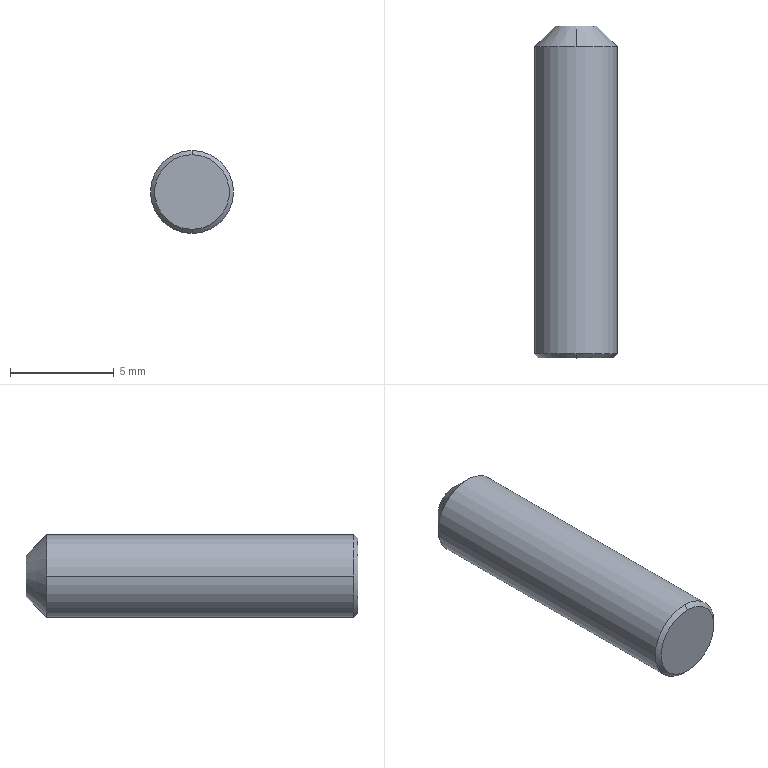Part | STEP file | 1 solid | 8 faces | box 4 x 16 x 4 mm | volume 195.583 mm3 | cone 4 | cylinder 2 | plane 2 | commonest cylinder face diameters 4 x2
STEP:
#1=CARTESIAN_POINT('',(0.,0.,0.));
#2=DIRECTION('',(0.,0.,1.));
#3=DIRECTION('',(1.,0.,0.));
#4=AXIS2_PLACEMENT_3D('',#1,#2,#3);
#5=CARTESIAN_POINT('',(0.,0.,-1.8));
#6=VERTEX_POINT('',#5);
#7=CARTESIAN_POINT('',(0.,0.,1.8));
#8=VERTEX_POINT('',#7);
#9=CARTESIAN_POINT('',(0.,0.,0.));
#10=DIRECTION('',(0.,-1.,0.));
#11=DIRECTION('',(0.,0.,1.));
#12=AXIS2_PLACEMENT_3D('',#9,#10,#11);
#13=CIRCLE('',#12,1.8);
#14=CARTESIAN_POINT('',(0.,0.,0.));
#15=DIRECTION('',(0.,1.,0.));
#16=DIRECTION('',(0.,0.,1.));
#17=AXIS2_PLACEMENT_3D('',#14,#15,#16);
#18=CONICAL_SURFACE('',#17,1.8,0.7854);
#19=CARTESIAN_POINT('',(6.283,0.));
#20=DIRECTION('',(-1.,0.));
#21=VECTOR('',#20,1.);
#22=LINE('',#19,#21);
#23=(GEOMETRIC_REPRESENTATION_CONTEXT(2)PARAMETRIC_REPRESENTATION_CONTEXT()REPRESENTATION_CONTEXT('',''));
#24=DEFINITIONAL_REPRESENTATION('',(#22),#23);
#25=PCURVE('',#18,#24);
#26=CARTESIAN_POINT('',(-1.822,0.,1.822));
#27=DIRECTION('',(0.,-1.,0.));
#28=DIRECTION('',(0.,0.,-1.));
#29=AXIS2_PLACEMENT_3D('',#26,#27,#28);
#30=PLANE('',#29);
#31=CARTESIAN_POINT('',(1.822,1.822));
#32=DIRECTION('',(-1.,0.));
#33=AXIS2_PLACEMENT_2D('',#31,#32);
#34=CIRCLE('',#33,1.8);
#35=(GEOMETRIC_REPRESENTATION_CONTEXT(2)PARAMETRIC_REPRESENTATION_CONTEXT()REPRESENTATION_CONTEXT('',''));
#36=DEFINITIONAL_REPRESENTATION('',(#34),#35);
#37=PCURVE('',#30,#36);
#38=SURFACE_CURVE('',#13,(#25,#37),.PCURVE_S1.);
#39=EDGE_CURVE('',#6,#8,#38,.T.);
#40=ORIENTED_EDGE('',*,*,#39,.F.);
#41=CARTESIAN_POINT('',(0.,0.2,-2.));
#42=VERTEX_POINT('',#41);
#43=CARTESIAN_POINT('',(0.,0.,-1.8));
#44=DIRECTION('',(0.,0.7071,-0.7071));
#45=VECTOR('',#44,1.);
#46=LINE('',#43,#45);
#47=CARTESIAN_POINT('',(3.142,0.));
#48=DIRECTION('',(0.,1.));
#49=VECTOR('',#48,1.);
#50=LINE('',#47,#49);
#51=(GEOMETRIC_REPRESENTATION_CONTEXT(2)PARAMETRIC_REPRESENTATION_CONTEXT()REPRESENTATION_CONTEXT('',''));
#52=DEFINITIONAL_REPRESENTATION('',(#50),#51);
#53=PCURVE('',#18,#52);
#54=CARTESIAN_POINT('',(0.,0.,0.));
#55=DIRECTION('',(0.,1.,0.));
#56=DIRECTION('',(0.,0.,1.));
#57=AXIS2_PLACEMENT_3D('',#54,#55,#56);
#58=CONICAL_SURFACE('',#57,1.8,0.7854);
#59=CARTESIAN_POINT('',(3.142,0.));
#60=DIRECTION('',(0.,1.));
#61=VECTOR('',#60,1.);
#62=LINE('',#59,#61);
#63=(GEOMETRIC_REPRESENTATION_CONTEXT(2)PARAMETRIC_REPRESENTATION_CONTEXT()REPRESENTATION_CONTEXT('',''));
#64=DEFINITIONAL_REPRESENTATION('',(#62),#63);
#65=PCURVE('',#58,#64);
#66=SURFACE_CURVE('',#46,(#53,#65),.PCURVE_S1.);
#67=EDGE_CURVE('',#6,#42,#66,.T.);
#68=ORIENTED_EDGE('',*,*,#67,.T.);
#69=CARTESIAN_POINT('',(2.,0.2,0.));
#70=VERTEX_POINT('',#69);
#71=CARTESIAN_POINT('',(0.,0.2,0.));
#72=DIRECTION('',(0.,1.,0.));
#73=DIRECTION('',(0.,0.,1.));
#74=AXIS2_PLACEMENT_3D('',#71,#72,#73);
#75=CIRCLE('',#74,2.);
#76=CARTESIAN_POINT('',(0.,0.2));
#77=DIRECTION('',(1.,0.));
#78=VECTOR('',#77,1.);
#79=LINE('',#76,#78);
#80=(GEOMETRIC_REPRESENTATION_CONTEXT(2)PARAMETRIC_REPRESENTATION_CONTEXT()REPRESENTATION_CONTEXT('',''));
#81=DEFINITIONAL_REPRESENTATION('',(#79),#80);
#82=PCURVE('',#18,#81);
#83=CARTESIAN_POINT('',(0.,15.,0.));
#84=DIRECTION('',(0.,-1.,0.));
#85=DIRECTION('',(1.,0.,0.));
#86=AXIS2_PLACEMENT_3D('',#83,#84,#85);
#87=CYLINDRICAL_SURFACE('',#86,2.);
#88=CARTESIAN_POINT('',(7.854,14.8));
#89=DIRECTION('',(-1.,0.));
#90=VECTOR('',#89,1.);
#91=LINE('',#88,#90);
#92=(GEOMETRIC_REPRESENTATION_CONTEXT(2)PARAMETRIC_REPRESENTATION_CONTEXT()REPRESENTATION_CONTEXT('',''));
#93=DEFINITIONAL_REPRESENTATION('',(#91),#92);
#94=PCURVE('',#87,#93);
#95=SURFACE_CURVE('',#75,(#82,#94),.PCURVE_S1.);
#96=EDGE_CURVE('',#70,#42,#95,.T.);
#97=ORIENTED_EDGE('',*,*,#96,.F.);
#98=CARTESIAN_POINT('',(0.,0.2,2.));
#99=VERTEX_POINT('',#98);
#100=CARTESIAN_POINT('',(0.,0.2,0.));
#101=DIRECTION('',(0.,1.,0.));
#102=DIRECTION('',(0.,0.,1.));
#103=AXIS2_PLACEMENT_3D('',#100,#101,#102);
#104=CIRCLE('',#103,2.);
#105=CARTESIAN_POINT('',(0.,0.2));
#106=DIRECTION('',(1.,0.));
#107=VECTOR('',#106,1.);
#108=LINE('',#105,#107);
#109=(GEOMETRIC_REPRESENTATION_CONTEXT(2)PARAMETRIC_REPRESENTATION_CONTEXT()REPRESENTATION_CONTEXT('',''));
#110=DEFINITIONAL_REPRESENTATION('',(#108),#109);
#111=PCURVE('',#18,#110);
#112=CARTESIAN_POINT('',(0.,15.,0.));
#113=DIRECTION('',(0.,-1.,0.));
#114=DIRECTION('',(1.,0.,0.));
#115=AXIS2_PLACEMENT_3D('',#112,#113,#114);
#116=CYLINDRICAL_SURFACE('',#115,2.);
#117=CARTESIAN_POINT('',(1.571,14.8));
#118=DIRECTION('',(-1.,0.));
#119=VECTOR('',#118,1.);
#120=LINE('',#117,#119);
#121=(GEOMETRIC_REPRESENTATION_CONTEXT(2)PARAMETRIC_REPRESENTATION_CONTEXT()REPRESENTATION_CONTEXT('',''));
#122=DEFINITIONAL_REPRESENTATION('',(#120),#121);
#123=PCURVE('',#116,#122);
#124=SURFACE_CURVE('',#104,(#111,#123),.PCURVE_S1.);
#125=EDGE_CURVE('',#99,#70,#124,.T.);
#126=ORIENTED_EDGE('',*,*,#125,.F.);
#127=CARTESIAN_POINT('',(0.,0.,1.8));
#128=DIRECTION('',(0.,0.7071,0.7071));
#129=VECTOR('',#128,1.);
#130=LINE('',#127,#129);
#131=CARTESIAN_POINT('',(0.,0.));
#132=DIRECTION('',(0.,1.));
#133=VECTOR('',#132,1.);
#134=LINE('',#131,#133);
#135=(GEOMETRIC_REPRESENTATION_CONTEXT(2)PARAMETRIC_REPRESENTATION_CONTEXT()REPRESENTATION_CONTEXT('',''));
#136=DEFINITIONAL_REPRESENTATION('',(#134),#135);
#137=PCURVE('',#18,#136);
#138=CARTESIAN_POINT('',(6.283,0.));
#139=DIRECTION('',(0.,1.));
#140=VECTOR('',#139,1.);
#141=LINE('',#138,#140);
#142=(GEOMETRIC_REPRESENTATION_CONTEXT(2)PARAMETRIC_REPRESENTATION_CONTEXT()REPRESENTATION_CONTEXT('',''));
#143=DEFINITIONAL_REPRESENTATION('',(#141),#142);
#144=PCURVE('',#58,#143);
#145=SURFACE_CURVE('',#130,(#137,#144),.PCURVE_S1.);
#146=EDGE_CURVE('',#8,#99,#145,.T.);
#147=ORIENTED_EDGE('',*,*,#146,.F.);
#148=EDGE_LOOP('',(#40,#68,#97,#126,#147));
#149=FACE_BOUND('',#148,.T.);
#150=ADVANCED_FACE('',(#149),#18,.T.);
#151=CARTESIAN_POINT('',(-2.,15.,0.));
#152=VERTEX_POINT('',#151);
#153=CARTESIAN_POINT('',(0.,15.,2.));
#154=VERTEX_POINT('',#153);
#155=CARTESIAN_POINT('',(0.,15.,0.));
#156=DIRECTION('',(0.,1.,0.));
#157=DIRECTION('',(0.,0.,-1.));
#158=AXIS2_PLACEMENT_3D('',#155,#156,#157);
#159=CIRCLE('',#158,2.);
#160=CARTESIAN_POINT('',(4.712,0.));
#161=DIRECTION('',(-1.,0.));
#162=VECTOR('',#161,1.);
#163=LINE('',#160,#162);
#164=(GEOMETRIC_REPRESENTATION_CONTEXT(2)PARAMETRIC_REPRESENTATION_CONTEXT()REPRESENTATION_CONTEXT('',''));
#165=DEFINITIONAL_REPRESENTATION('',(#163),#164);
#166=PCURVE('',#116,#165);
#167=CARTESIAN_POINT('',(0.,16.,0.));
#168=DIRECTION('',(0.,-1.,0.));
#169=DIRECTION('',(0.,0.,-1.));
#170=AXIS2_PLACEMENT_3D('',#167,#168,#169);
#171=CONICAL_SURFACE('',#170,1.,0.7854);
#172=CARTESIAN_POINT('',(6.283,1.));
#173=DIRECTION('',(-1.,0.));
#174=VECTOR('',#173,1.);
#175=LINE('',#172,#174);
#176=(GEOMETRIC_REPRESENTATION_CONTEXT(2)PARAMETRIC_REPRESENTATION_CONTEXT()REPRESENTATION_CONTEXT('',''));
#177=DEFINITIONAL_REPRESENTATION('',(#175),#176);
#178=PCURVE('',#171,#177);
#179=SURFACE_CURVE('',#159,(#166,#178),.PCURVE_S1.);
#180=EDGE_CURVE('',#152,#154,#179,.T.);
#181=ORIENTED_EDGE('',*,*,#180,.F.);
#182=CARTESIAN_POINT('',(-2.,0.2,0.));
#183=VERTEX_POINT('',#182);
#184=CARTESIAN_POINT('',(-2.,15.,0.));
#185=DIRECTION('',(0.,-1.,0.));
#186=VECTOR('',#185,1.);
#187=LINE('',#184,#186);
#188=CARTESIAN_POINT('',(3.142,0.));
#189=DIRECTION('',(0.,1.));
#190=VECTOR('',#189,1.);
#191=LINE('',#188,#190);
#192=(GEOMETRIC_REPRESENTATION_CONTEXT(2)PARAMETRIC_REPRESENTATION_CONTEXT()REPRESENTATION_CONTEXT('',''));
#193=DEFINITIONAL_REPRESENTATION('',(#191),#192);
#194=PCURVE('',#116,#193);
#195=CARTESIAN_POINT('',(3.142,0.));
#196=DIRECTION('',(0.,1.));
#197=VECTOR('',#196,1.);
#198=LINE('',#195,#197);
#199=(GEOMETRIC_REPRESENTATION_CONTEXT(2)PARAMETRIC_REPRESENTATION_CONTEXT()REPRESENTATION_CONTEXT('',''));
#200=DEFINITIONAL_REPRESENTATION('',(#198),#199);
#201=PCURVE('',#87,#200);
#202=SURFACE_CURVE('',#187,(#194,#201),.PCURVE_S1.);
#203=EDGE_CURVE('',#152,#183,#202,.T.);
#204=ORIENTED_EDGE('',*,*,#203,.T.);
#205=CARTESIAN_POINT('',(0.,0.2,0.));
#206=DIRECTION('',(0.,1.,0.));
#207=DIRECTION('',(0.,0.,1.));
#208=AXIS2_PLACEMENT_3D('',#205,#206,#207);
#209=CIRCLE('',#208,2.);
#210=CARTESIAN_POINT('',(7.854,14.8));
#211=DIRECTION('',(-1.,0.));
#212=VECTOR('',#211,1.);
#213=LINE('',#210,#212);
#214=(GEOMETRIC_REPRESENTATION_CONTEXT(2)PARAMETRIC_REPRESENTATION_CONTEXT()REPRESENTATION_CONTEXT('',''));
#215=DEFINITIONAL_REPRESENTATION('',(#213),#214);
#216=PCURVE('',#116,#215);
#217=CARTESIAN_POINT('',(0.,0.2));
#218=DIRECTION('',(1.,0.));
#219=VECTOR('',#218,1.);
#220=LINE('',#217,#219);
#221=(GEOMETRIC_REPRESENTATION_CONTEXT(2)PARAMETRIC_REPRESENTATION_CONTEXT()REPRESENTATION_CONTEXT('',''));
#222=DEFINITIONAL_REPRESENTATION('',(#220),#221);
#223=PCURVE('',#58,#222);
#224=SURFACE_CURVE('',#209,(#216,#223),.PCURVE_S1.);
#225=EDGE_CURVE('',#183,#99,#224,.T.);
#226=ORIENTED_EDGE('',*,*,#225,.T.);
#227=ORIENTED_EDGE('',*,*,#125,.T.);
#228=CARTESIAN_POINT('',(2.,15.,0.));
#229=VERTEX_POINT('',#228);
#230=CARTESIAN_POINT('',(2.,15.,0.));
#231=DIRECTION('',(0.,-1.,0.));
#232=VECTOR('',#231,1.);
#233=LINE('',#230,#232);
#234=CARTESIAN_POINT('',(0.,0.));
#235=DIRECTION('',(0.,1.));
#236=VECTOR('',#235,1.);
#237=LINE('',#234,#236);
#238=(GEOMETRIC_REPRESENTATION_CONTEXT(2)PARAMETRIC_REPRESENTATION_CONTEXT()REPRESENTATION_CONTEXT('',''));
#239=DEFINITIONAL_REPRESENTATION('',(#237),#238);
#240=PCURVE('',#116,#239);
#241=CARTESIAN_POINT('',(6.283,0.));
#242=DIRECTION('',(0.,1.));
#243=VECTOR('',#242,1.);
#244=LINE('',#241,#243);
#245=(GEOMETRIC_REPRESENTATION_CONTEXT(2)PARAMETRIC_REPRESENTATION_CONTEXT()REPRESENTATION_CONTEXT('',''));
#246=DEFINITIONAL_REPRESENTATION('',(#244),#245);
#247=PCURVE('',#87,#246);
#248=SURFACE_CURVE('',#233,(#240,#247),.PCURVE_S1.);
#249=EDGE_CURVE('',#229,#70,#248,.T.);
#250=ORIENTED_EDGE('',*,*,#249,.F.);
#251=CARTESIAN_POINT('',(0.,15.,0.));
#252=DIRECTION('',(0.,1.,0.));
#253=DIRECTION('',(0.,0.,-1.));
#254=AXIS2_PLACEMENT_3D('',#251,#252,#253);
#255=CIRCLE('',#254,2.);
#256=CARTESIAN_POINT('',(4.712,0.));
#257=DIRECTION('',(-1.,0.));
#258=VECTOR('',#257,1.);
#259=LINE('',#256,#258);
#260=(GEOMETRIC_REPRESENTATION_CONTEXT(2)PARAMETRIC_REPRESENTATION_CONTEXT()REPRESENTATION_CONTEXT('',''));
#261=DEFINITIONAL_REPRESENTATION('',(#259),#260);
#262=PCURVE('',#116,#261);
#263=CARTESIAN_POINT('',(0.,16.,0.));
#264=DIRECTION('',(0.,-1.,0.));
#265=DIRECTION('',(0.,0.,-1.));
#266=AXIS2_PLACEMENT_3D('',#263,#264,#265);
#267=CONICAL_SURFACE('',#266,1.,0.7854);
#268=CARTESIAN_POINT('',(6.283,1.));
#269=DIRECTION('',(-1.,0.));
#270=VECTOR('',#269,1.);
#271=LINE('',#268,#270);
#272=(GEOMETRIC_REPRESENTATION_CONTEXT(2)PARAMETRIC_REPRESENTATION_CONTEXT()REPRESENTATION_CONTEXT('',''));
#273=DEFINITIONAL_REPRESENTATION('',(#271),#272);
#274=PCURVE('',#267,#273);
#275=SURFACE_CURVE('',#255,(#262,#274),.PCURVE_S1.);
#276=EDGE_CURVE('',#154,#229,#275,.T.);
#277=ORIENTED_EDGE('',*,*,#276,.F.);
#278=EDGE_LOOP('',(#181,#204,#226,#227,#250,#277));
#279=FACE_BOUND('',#278,.T.);
#280=ADVANCED_FACE('',(#279),#116,.T.);
#281=CARTESIAN_POINT('',(0.,16.,1.));
#282=VERTEX_POINT('',#281);
#283=CARTESIAN_POINT('',(0.,16.,-1.));
#284=VERTEX_POINT('',#283);
#285=CARTESIAN_POINT('',(0.,16.,0.));
#286=DIRECTION('',(0.,1.,0.));
#287=DIRECTION('',(0.,0.,-1.));
#288=AXIS2_PLACEMENT_3D('',#285,#286,#287);
#289=CIRCLE('',#288,1.);
#290=CARTESIAN_POINT('',(6.283,0.));
#291=DIRECTION('',(-1.,0.));
#292=VECTOR('',#291,1.);
#293=LINE('',#290,#292);
#294=(GEOMETRIC_REPRESENTATION_CONTEXT(2)PARAMETRIC_REPRESENTATION_CONTEXT()REPRESENTATION_CONTEXT('',''));
#295=DEFINITIONAL_REPRESENTATION('',(#293),#294);
#296=PCURVE('',#267,#295);
#297=CARTESIAN_POINT('',(-1.012,16.,-1.012));
#298=DIRECTION('',(0.,1.,0.));
#299=DIRECTION('',(0.,0.,1.));
#300=AXIS2_PLACEMENT_3D('',#297,#298,#299);
#301=PLANE('',#300);
#302=CARTESIAN_POINT('',(1.012,1.012));
#303=DIRECTION('',(-1.,0.));
#304=AXIS2_PLACEMENT_2D('',#302,#303);
#305=CIRCLE('',#304,1.);
#306=(GEOMETRIC_REPRESENTATION_CONTEXT(2)PARAMETRIC_REPRESENTATION_CONTEXT()REPRESENTATION_CONTEXT('',''));
#307=DEFINITIONAL_REPRESENTATION('',(#305),#306);
#308=PCURVE('',#301,#307);
#309=SURFACE_CURVE('',#289,(#296,#308),.PCURVE_S1.);
#310=EDGE_CURVE('',#282,#284,#309,.T.);
#311=ORIENTED_EDGE('',*,*,#310,.F.);
#312=CARTESIAN_POINT('',(0.,16.,1.));
#313=DIRECTION('',(0.,-0.7071,0.7071));
#314=VECTOR('',#313,1.);
#315=LINE('',#312,#314);
#316=CARTESIAN_POINT('',(3.142,0.));
#317=DIRECTION('',(0.,1.));
#318=VECTOR('',#317,1.);
#319=LINE('',#316,#318);
#320=(GEOMETRIC_REPRESENTATION_CONTEXT(2)PARAMETRIC_REPRESENTATION_CONTEXT()REPRESENTATION_CONTEXT('',''));
#321=DEFINITIONAL_REPRESENTATION('',(#319),#320);
#322=PCURVE('',#267,#321);
#323=CARTESIAN_POINT('',(3.142,0.));
#324=DIRECTION('',(0.,1.));
#325=VECTOR('',#324,1.);
#326=LINE('',#323,#325);
#327=(GEOMETRIC_REPRESENTATION_CONTEXT(2)PARAMETRIC_REPRESENTATION_CONTEXT()REPRESENTATION_CONTEXT('',''));
#328=DEFINITIONAL_REPRESENTATION('',(#326),#327);
#329=PCURVE('',#171,#328);
#330=SURFACE_CURVE('',#315,(#322,#329),.PCURVE_S1.);
#331=EDGE_CURVE('',#282,#154,#330,.T.);
#332=ORIENTED_EDGE('',*,*,#331,.T.);
#333=ORIENTED_EDGE('',*,*,#276,.T.);
#334=CARTESIAN_POINT('',(0.,15.,-2.));
#335=VERTEX_POINT('',#334);
#336=CARTESIAN_POINT('',(0.,15.,0.));
#337=DIRECTION('',(0.,1.,0.));
#338=DIRECTION('',(0.,0.,-1.));
#339=AXIS2_PLACEMENT_3D('',#336,#337,#338);
#340=CIRCLE('',#339,2.);
#341=CARTESIAN_POINT('',(6.283,1.));
#342=DIRECTION('',(-1.,0.));
#343=VECTOR('',#342,1.);
#344=LINE('',#341,#343);
#345=(GEOMETRIC_REPRESENTATION_CONTEXT(2)PARAMETRIC_REPRESENTATION_CONTEXT()REPRESENTATION_CONTEXT('',''));
#346=DEFINITIONAL_REPRESENTATION('',(#344),#345);
#347=PCURVE('',#267,#346);
#348=CARTESIAN_POINT('',(10.996,0.));
#349=DIRECTION('',(-1.,0.));
#350=VECTOR('',#349,1.);
#351=LINE('',#348,#350);
#352=(GEOMETRIC_REPRESENTATION_CONTEXT(2)PARAMETRIC_REPRESENTATION_CONTEXT()REPRESENTATION_CONTEXT('',''));
#353=DEFINITIONAL_REPRESENTATION('',(#351),#352);
#354=PCURVE('',#87,#353);
#355=SURFACE_CURVE('',#340,(#347,#354),.PCURVE_S1.);
#356=EDGE_CURVE('',#229,#335,#355,.T.);
#357=ORIENTED_EDGE('',*,*,#356,.T.);
#358=CARTESIAN_POINT('',(0.,16.,-1.));
#359=DIRECTION('',(0.,-0.7071,-0.7071));
#360=VECTOR('',#359,1.);
#361=LINE('',#358,#360);
#362=CARTESIAN_POINT('',(0.,0.));
#363=DIRECTION('',(0.,1.));
#364=VECTOR('',#363,1.);
#365=LINE('',#362,#364);
#366=(GEOMETRIC_REPRESENTATION_CONTEXT(2)PARAMETRIC_REPRESENTATION_CONTEXT()REPRESENTATION_CONTEXT('',''));
#367=DEFINITIONAL_REPRESENTATION('',(#365),#366);
#368=PCURVE('',#267,#367);
#369=CARTESIAN_POINT('',(6.283,0.));
#370=DIRECTION('',(0.,1.));
#371=VECTOR('',#370,1.);
#372=LINE('',#369,#371);
#373=(GEOMETRIC_REPRESENTATION_CONTEXT(2)PARAMETRIC_REPRESENTATION_CONTEXT()REPRESENTATION_CONTEXT('',''));
#374=DEFINITIONAL_REPRESENTATION('',(#372),#373);
#375=PCURVE('',#171,#374);
#376=SURFACE_CURVE('',#361,(#368,#375),.PCURVE_S1.);
#377=EDGE_CURVE('',#284,#335,#376,.T.);
#378=ORIENTED_EDGE('',*,*,#377,.F.);
#379=EDGE_LOOP('',(#311,#332,#333,#357,#378));
#380=FACE_BOUND('',#379,.T.);
#381=ADVANCED_FACE('',(#380),#267,.T.);
#382=ORIENTED_EDGE('',*,*,#67,.F.);
#383=CARTESIAN_POINT('',(0.,0.,0.));
#384=DIRECTION('',(0.,-1.,0.));
#385=DIRECTION('',(0.,0.,1.));
#386=AXIS2_PLACEMENT_3D('',#383,#384,#385);
#387=CIRCLE('',#386,1.8);
#388=CARTESIAN_POINT('',(6.283,0.));
#389=DIRECTION('',(-1.,0.));
#390=VECTOR('',#389,1.);
#391=LINE('',#388,#390);
#392=(GEOMETRIC_REPRESENTATION_CONTEXT(2)PARAMETRIC_REPRESENTATION_CONTEXT()REPRESENTATION_CONTEXT('',''));
#393=DEFINITIONAL_REPRESENTATION('',(#391),#392);
#394=PCURVE('',#58,#393);
#395=CARTESIAN_POINT('',(1.822,1.822));
#396=DIRECTION('',(-1.,0.));
#397=AXIS2_PLACEMENT_2D('',#395,#396);
#398=CIRCLE('',#397,1.8);
#399=(GEOMETRIC_REPRESENTATION_CONTEXT(2)PARAMETRIC_REPRESENTATION_CONTEXT()REPRESENTATION_CONTEXT('',''));
#400=DEFINITIONAL_REPRESENTATION('',(#398),#399);
#401=PCURVE('',#30,#400);
#402=SURFACE_CURVE('',#387,(#394,#401),.PCURVE_S1.);
#403=EDGE_CURVE('',#8,#6,#402,.T.);
#404=ORIENTED_EDGE('',*,*,#403,.F.);
#405=ORIENTED_EDGE('',*,*,#146,.T.);
#406=ORIENTED_EDGE('',*,*,#225,.F.);
#407=CARTESIAN_POINT('',(0.,0.2,0.));
#408=DIRECTION('',(0.,1.,0.));
#409=DIRECTION('',(0.,0.,1.));
#410=AXIS2_PLACEMENT_3D('',#407,#408,#409);
#411=CIRCLE('',#410,2.);
#412=CARTESIAN_POINT('',(0.,0.2));
#413=DIRECTION('',(1.,0.));
#414=VECTOR('',#413,1.);
#415=LINE('',#412,#414);
#416=(GEOMETRIC_REPRESENTATION_CONTEXT(2)PARAMETRIC_REPRESENTATION_CONTEXT()REPRESENTATION_CONTEXT('',''));
#417=DEFINITIONAL_REPRESENTATION('',(#415),#416);
#418=PCURVE('',#58,#417);
#419=CARTESIAN_POINT('',(7.854,14.8));
#420=DIRECTION('',(-1.,0.));
#421=VECTOR('',#420,1.);
#422=LINE('',#419,#421);
#423=(GEOMETRIC_REPRESENTATION_CONTEXT(2)PARAMETRIC_REPRESENTATION_CONTEXT()REPRESENTATION_CONTEXT('',''));
#424=DEFINITIONAL_REPRESENTATION('',(#422),#423);
#425=PCURVE('',#87,#424);
#426=SURFACE_CURVE('',#411,(#418,#425),.PCURVE_S1.);
#427=EDGE_CURVE('',#42,#183,#426,.T.);
#428=ORIENTED_EDGE('',*,*,#427,.F.);
#429=EDGE_LOOP('',(#382,#404,#405,#406,#428));
#430=FACE_BOUND('',#429,.T.);
#431=ADVANCED_FACE('',(#430),#58,.T.);
#432=ORIENTED_EDGE('',*,*,#403,.T.);
#433=ORIENTED_EDGE('',*,*,#39,.T.);
#434=EDGE_LOOP('',(#432,#433));
#435=FACE_BOUND('',#434,.T.);
#436=ADVANCED_FACE('',(#435),#30,.T.);
#437=ORIENTED_EDGE('',*,*,#203,.F.);
#438=CARTESIAN_POINT('',(0.,15.,0.));
#439=DIRECTION('',(0.,1.,0.));
#440=DIRECTION('',(0.,0.,-1.));
#441=AXIS2_PLACEMENT_3D('',#438,#439,#440);
#442=CIRCLE('',#441,2.);
#443=CARTESIAN_POINT('',(4.712,0.));
#444=DIRECTION('',(-1.,0.));
#445=VECTOR('',#444,1.);
#446=LINE('',#443,#445);
#447=(GEOMETRIC_REPRESENTATION_CONTEXT(2)PARAMETRIC_REPRESENTATION_CONTEXT()REPRESENTATION_CONTEXT('',''));
#448=DEFINITIONAL_REPRESENTATION('',(#446),#447);
#449=PCURVE('',#87,#448);
#450=CARTESIAN_POINT('',(6.283,1.));
#451=DIRECTION('',(-1.,0.));
#452=VECTOR('',#451,1.);
#453=LINE('',#450,#452);
#454=(GEOMETRIC_REPRESENTATION_CONTEXT(2)PARAMETRIC_REPRESENTATION_CONTEXT()REPRESENTATION_CONTEXT('',''));
#455=DEFINITIONAL_REPRESENTATION('',(#453),#454);
#456=PCURVE('',#171,#455);
#457=SURFACE_CURVE('',#442,(#449,#456),.PCURVE_S1.);
#458=EDGE_CURVE('',#335,#152,#457,.T.);
#459=ORIENTED_EDGE('',*,*,#458,.F.);
#460=ORIENTED_EDGE('',*,*,#356,.F.);
#461=ORIENTED_EDGE('',*,*,#249,.T.);
#462=ORIENTED_EDGE('',*,*,#96,.T.);
#463=ORIENTED_EDGE('',*,*,#427,.T.);
#464=EDGE_LOOP('',(#437,#459,#460,#461,#462,#463));
#465=FACE_BOUND('',#464,.T.);
#466=ADVANCED_FACE('',(#465),#87,.T.);
#467=ORIENTED_EDGE('',*,*,#331,.F.);
#468=CARTESIAN_POINT('',(0.,16.,0.));
#469=DIRECTION('',(0.,1.,0.));
#470=DIRECTION('',(0.,0.,-1.));
#471=AXIS2_PLACEMENT_3D('',#468,#469,#470);
#472=CIRCLE('',#471,1.);
#473=CARTESIAN_POINT('',(6.283,0.));
#474=DIRECTION('',(-1.,0.));
#475=VECTOR('',#474,1.);
#476=LINE('',#473,#475);
#477=(GEOMETRIC_REPRESENTATION_CONTEXT(2)PARAMETRIC_REPRESENTATION_CONTEXT()REPRESENTATION_CONTEXT('',''));
#478=DEFINITIONAL_REPRESENTATION('',(#476),#477);
#479=PCURVE('',#171,#478);
#480=CARTESIAN_POINT('',(1.012,1.012));
#481=DIRECTION('',(-1.,0.));
#482=AXIS2_PLACEMENT_2D('',#480,#481);
#483=CIRCLE('',#482,1.);
#484=(GEOMETRIC_REPRESENTATION_CONTEXT(2)PARAMETRIC_REPRESENTATION_CONTEXT()REPRESENTATION_CONTEXT('',''));
#485=DEFINITIONAL_REPRESENTATION('',(#483),#484);
#486=PCURVE('',#301,#485);
#487=SURFACE_CURVE('',#472,(#479,#486),.PCURVE_S1.);
#488=EDGE_CURVE('',#284,#282,#487,.T.);
#489=ORIENTED_EDGE('',*,*,#488,.F.);
#490=ORIENTED_EDGE('',*,*,#377,.T.);
#491=ORIENTED_EDGE('',*,*,#458,.T.);
#492=ORIENTED_EDGE('',*,*,#180,.T.);
#493=EDGE_LOOP('',(#467,#489,#490,#491,#492));
#494=FACE_BOUND('',#493,.T.);
#495=ADVANCED_FACE('',(#494),#171,.T.);
#496=ORIENTED_EDGE('',*,*,#488,.T.);
#497=ORIENTED_EDGE('',*,*,#310,.T.);
#498=EDGE_LOOP('',(#496,#497));
#499=FACE_BOUND('',#498,.T.);
#500=ADVANCED_FACE('',(#499),#301,.T.);
#501=CLOSED_SHELL('',(#150,#280,#381,#431,#436,#466,#495,#500));
#502=MANIFOLD_SOLID_BREP('',#501);
#503=(LENGTH_UNIT()NAMED_UNIT(*)SI_UNIT(.MILLI.,.METRE.));
#504=UNCERTAINTY_MEASURE_WITH_UNIT(LENGTH_MEASURE(0.0000001),#503,'','');
#505=(NAMED_UNIT(*)PLANE_ANGLE_UNIT()SI_UNIT($,.RADIAN.));
#506=(NAMED_UNIT(*)SI_UNIT($,.STERADIAN.)SOLID_ANGLE_UNIT());
#507=(GEOMETRIC_REPRESENTATION_CONTEXT(3)GLOBAL_UNCERTAINTY_ASSIGNED_CONTEXT((#504))GLOBAL_UNIT_ASSIGNED_CONTEXT((#503,#505,#506))REPRESENTATION_CONTEXT('',''));
#508=ADVANCED_BREP_SHAPE_REPRESENTATION('',(#4,#502),#507);